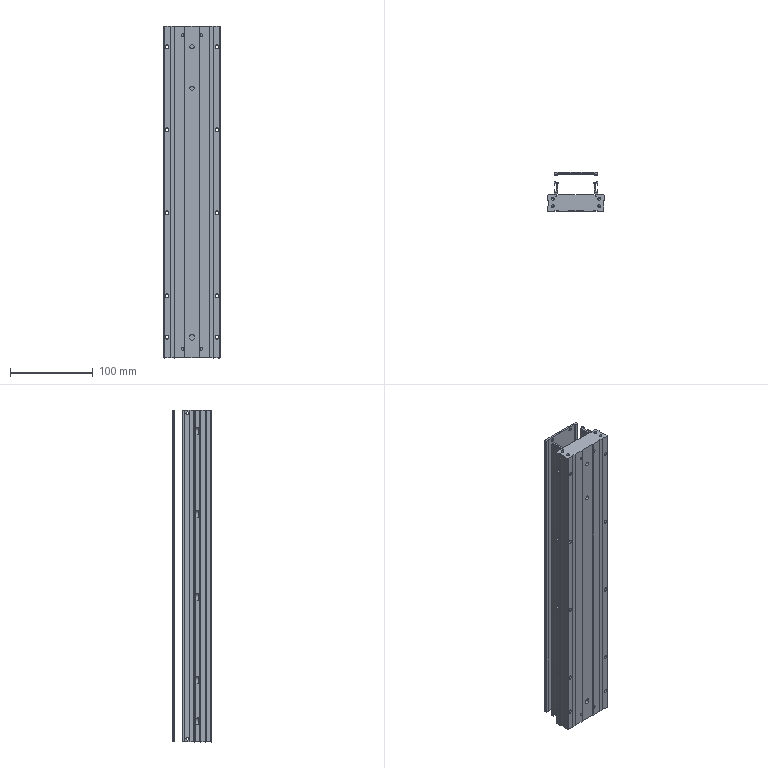Part | SolidWorks | features BaseBody 2 | 2 solids | 305 faces | box 68 x 47 x 400 mm | volume 601851 mm3 | plane 184 | cylinder 87 | cone 34 | commonest cylinder face diameters 3.3 x24 4.4 x20 8 x10 0.6 x9 3.4 x8 3.5 x8